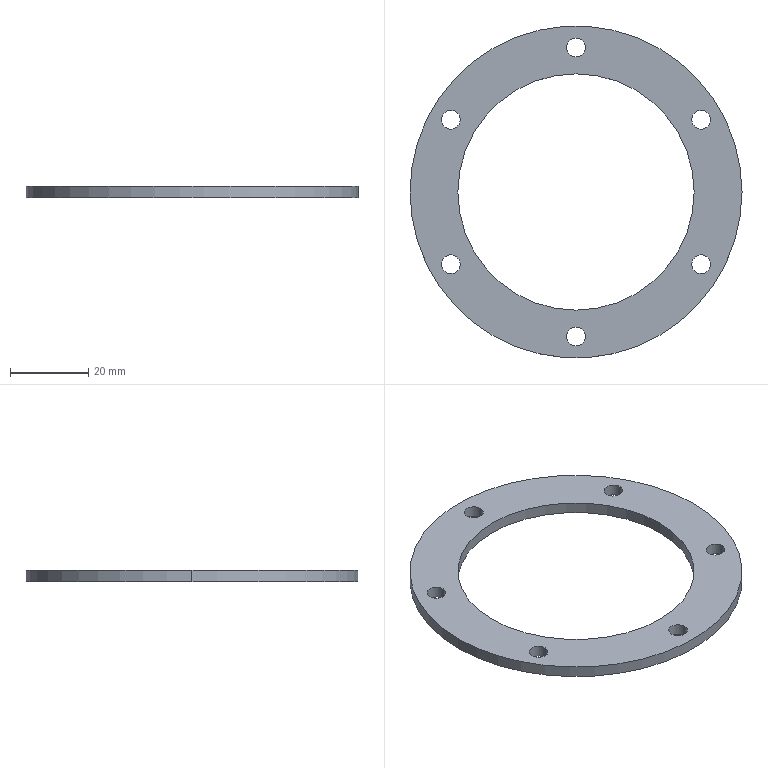Part | SolidWorks | features Extrusion 1, ICE 1 | 1 solid | 18 faces | box 85 x 85 x 3 mm | volume 8074 mm3 | cylinder 16 | plane 2 | commonest cylinder face diameters 4.8 x12 60.5 x2 85 x2
STEP:
#1=CARTESIAN_POINT('',(-34.443,18.5,0.));
#2=VERTEX_POINT('',#1);
#3=CARTESIAN_POINT('',(-29.643,18.5,0.));
#4=VERTEX_POINT('',#3);
#5=CARTESIAN_POINT('',(-32.043,18.5,0.));
#6=DIRECTION('',(0.,0.,1.));
#7=DIRECTION('',(1.,0.,0.));
#8=AXIS2_PLACEMENT_3D('',#5,#6,#7);
#9=CIRCLE('',#8,2.4);
#10=EDGE_CURVE('',#2,#4,#9,.T.);
#11=ORIENTED_EDGE('',*,*,#10,.F.);
#12=CARTESIAN_POINT('',(-34.443,18.5,3.));
#13=VERTEX_POINT('',#12);
#14=CARTESIAN_POINT('',(-34.443,18.5,0.));
#15=DIRECTION('',(0.,0.,1.));
#16=VECTOR('',#15,1000.);
#17=LINE('',#14,#16);
#18=EDGE_CURVE('',#2,#13,#17,.T.);
#19=ORIENTED_EDGE('',*,*,#18,.T.);
#20=CARTESIAN_POINT('',(-29.643,18.5,3.));
#21=VERTEX_POINT('',#20);
#22=CARTESIAN_POINT('',(-32.043,18.5,3.));
#23=DIRECTION('',(0.,0.,1.));
#24=DIRECTION('',(1.,0.,0.));
#25=AXIS2_PLACEMENT_3D('',#22,#23,#24);
#26=CIRCLE('',#25,2.4);
#27=EDGE_CURVE('',#13,#21,#26,.T.);
#28=ORIENTED_EDGE('',*,*,#27,.T.);
#29=CARTESIAN_POINT('',(-29.643,18.5,0.));
#30=DIRECTION('',(0.,0.,1.));
#31=VECTOR('',#30,1000.);
#32=LINE('',#29,#31);
#33=EDGE_CURVE('',#4,#21,#32,.T.);
#34=ORIENTED_EDGE('',*,*,#33,.F.);
#35=EDGE_LOOP('',(#11,#19,#28,#34));
#36=FACE_OUTER_BOUND('',#35,.T.);
#37=CARTESIAN_POINT('',(-32.043,18.5,0.));
#38=DIRECTION('',(0.,0.,1.));
#39=DIRECTION('',(1.,0.,0.));
#40=AXIS2_PLACEMENT_3D('',#37,#38,#39);
#41=CYLINDRICAL_SURFACE('',#40,2.4);
#42=ADVANCED_FACE('',(#36),#41,.F.);
#43=CARTESIAN_POINT('',(-34.443,-18.5,0.));
#44=VERTEX_POINT('',#43);
#45=CARTESIAN_POINT('',(-29.643,-18.5,0.));
#46=VERTEX_POINT('',#45);
#47=CARTESIAN_POINT('',(-32.043,-18.5,0.));
#48=DIRECTION('',(0.,0.,1.));
#49=DIRECTION('',(1.,0.,0.));
#50=AXIS2_PLACEMENT_3D('',#47,#48,#49);
#51=CIRCLE('',#50,2.4);
#52=EDGE_CURVE('',#44,#46,#51,.T.);
#53=ORIENTED_EDGE('',*,*,#52,.F.);
#54=CARTESIAN_POINT('',(-34.443,-18.5,3.));
#55=VERTEX_POINT('',#54);
#56=CARTESIAN_POINT('',(-34.443,-18.5,0.));
#57=DIRECTION('',(0.,0.,1.));
#58=VECTOR('',#57,1000.);
#59=LINE('',#56,#58);
#60=EDGE_CURVE('',#44,#55,#59,.T.);
#61=ORIENTED_EDGE('',*,*,#60,.T.);
#62=CARTESIAN_POINT('',(-29.643,-18.5,3.));
#63=VERTEX_POINT('',#62);
#64=CARTESIAN_POINT('',(-32.043,-18.5,3.));
#65=DIRECTION('',(0.,0.,1.));
#66=DIRECTION('',(1.,0.,0.));
#67=AXIS2_PLACEMENT_3D('',#64,#65,#66);
#68=CIRCLE('',#67,2.4);
#69=EDGE_CURVE('',#55,#63,#68,.T.);
#70=ORIENTED_EDGE('',*,*,#69,.T.);
#71=CARTESIAN_POINT('',(-29.643,-18.5,0.));
#72=DIRECTION('',(0.,0.,1.));
#73=VECTOR('',#72,1000.);
#74=LINE('',#71,#73);
#75=EDGE_CURVE('',#46,#63,#74,.T.);
#76=ORIENTED_EDGE('',*,*,#75,.F.);
#77=EDGE_LOOP('',(#53,#61,#70,#76));
#78=FACE_OUTER_BOUND('',#77,.T.);
#79=CARTESIAN_POINT('',(-32.043,-18.5,0.));
#80=DIRECTION('',(0.,0.,1.));
#81=DIRECTION('',(1.,0.,0.));
#82=AXIS2_PLACEMENT_3D('',#79,#80,#81);
#83=CYLINDRICAL_SURFACE('',#82,2.4);
#84=ADVANCED_FACE('',(#78),#83,.F.);
#85=CARTESIAN_POINT('',(-2.4,-37.,0.));
#86=VERTEX_POINT('',#85);
#87=CARTESIAN_POINT('',(2.4,-37.,0.));
#88=VERTEX_POINT('',#87);
#89=CARTESIAN_POINT('',(0.,-37.,0.));
#90=DIRECTION('',(0.,0.,1.));
#91=DIRECTION('',(1.,0.,0.));
#92=AXIS2_PLACEMENT_3D('',#89,#90,#91);
#93=CIRCLE('',#92,2.4);
#94=EDGE_CURVE('',#86,#88,#93,.T.);
#95=ORIENTED_EDGE('',*,*,#94,.F.);
#96=CARTESIAN_POINT('',(-2.4,-37.,3.));
#97=VERTEX_POINT('',#96);
#98=CARTESIAN_POINT('',(-2.4,-37.,0.));
#99=DIRECTION('',(0.,0.,1.));
#100=VECTOR('',#99,1000.);
#101=LINE('',#98,#100);
#102=EDGE_CURVE('',#86,#97,#101,.T.);
#103=ORIENTED_EDGE('',*,*,#102,.T.);
#104=CARTESIAN_POINT('',(2.4,-37.,3.));
#105=VERTEX_POINT('',#104);
#106=CARTESIAN_POINT('',(0.,-37.,3.));
#107=DIRECTION('',(0.,0.,1.));
#108=DIRECTION('',(1.,0.,0.));
#109=AXIS2_PLACEMENT_3D('',#106,#107,#108);
#110=CIRCLE('',#109,2.4);
#111=EDGE_CURVE('',#97,#105,#110,.T.);
#112=ORIENTED_EDGE('',*,*,#111,.T.);
#113=CARTESIAN_POINT('',(2.4,-37.,0.));
#114=DIRECTION('',(0.,0.,1.));
#115=VECTOR('',#114,1000.);
#116=LINE('',#113,#115);
#117=EDGE_CURVE('',#88,#105,#116,.T.);
#118=ORIENTED_EDGE('',*,*,#117,.F.);
#119=EDGE_LOOP('',(#95,#103,#112,#118));
#120=FACE_OUTER_BOUND('',#119,.T.);
#121=CARTESIAN_POINT('',(0.,-37.,0.));
#122=DIRECTION('',(0.,0.,1.));
#123=DIRECTION('',(1.,0.,0.));
#124=AXIS2_PLACEMENT_3D('',#121,#122,#123);
#125=CYLINDRICAL_SURFACE('',#124,2.4);
#126=ADVANCED_FACE('',(#120),#125,.F.);
#127=CARTESIAN_POINT('',(29.643,-18.5,0.));
#128=VERTEX_POINT('',#127);
#129=CARTESIAN_POINT('',(34.443,-18.5,0.));
#130=VERTEX_POINT('',#129);
#131=CARTESIAN_POINT('',(32.043,-18.5,0.));
#132=DIRECTION('',(0.,0.,1.));
#133=DIRECTION('',(1.,0.,0.));
#134=AXIS2_PLACEMENT_3D('',#131,#132,#133);
#135=CIRCLE('',#134,2.4);
#136=EDGE_CURVE('',#128,#130,#135,.T.);
#137=ORIENTED_EDGE('',*,*,#136,.F.);
#138=CARTESIAN_POINT('',(29.643,-18.5,3.));
#139=VERTEX_POINT('',#138);
#140=CARTESIAN_POINT('',(29.643,-18.5,0.));
#141=DIRECTION('',(0.,0.,1.));
#142=VECTOR('',#141,1000.);
#143=LINE('',#140,#142);
#144=EDGE_CURVE('',#128,#139,#143,.T.);
#145=ORIENTED_EDGE('',*,*,#144,.T.);
#146=CARTESIAN_POINT('',(34.443,-18.5,3.));
#147=VERTEX_POINT('',#146);
#148=CARTESIAN_POINT('',(32.043,-18.5,3.));
#149=DIRECTION('',(0.,0.,1.));
#150=DIRECTION('',(1.,0.,0.));
#151=AXIS2_PLACEMENT_3D('',#148,#149,#150);
#152=CIRCLE('',#151,2.4);
#153=EDGE_CURVE('',#139,#147,#152,.T.);
#154=ORIENTED_EDGE('',*,*,#153,.T.);
#155=CARTESIAN_POINT('',(34.443,-18.5,0.));
#156=DIRECTION('',(0.,0.,1.));
#157=VECTOR('',#156,1000.);
#158=LINE('',#155,#157);
#159=EDGE_CURVE('',#130,#147,#158,.T.);
#160=ORIENTED_EDGE('',*,*,#159,.F.);
#161=EDGE_LOOP('',(#137,#145,#154,#160));
#162=FACE_OUTER_BOUND('',#161,.T.);
#163=CARTESIAN_POINT('',(32.043,-18.5,0.));
#164=DIRECTION('',(0.,0.,1.));
#165=DIRECTION('',(1.,0.,0.));
#166=AXIS2_PLACEMENT_3D('',#163,#164,#165);
#167=CYLINDRICAL_SURFACE('',#166,2.4);
#168=ADVANCED_FACE('',(#162),#167,.F.);
#169=CARTESIAN_POINT('',(29.643,18.5,0.));
#170=VERTEX_POINT('',#169);
#171=CARTESIAN_POINT('',(34.443,18.5,0.));
#172=VERTEX_POINT('',#171);
#173=CARTESIAN_POINT('',(32.043,18.5,0.));
#174=DIRECTION('',(0.,0.,1.));
#175=DIRECTION('',(1.,0.,0.));
#176=AXIS2_PLACEMENT_3D('',#173,#174,#175);
#177=CIRCLE('',#176,2.4);
#178=EDGE_CURVE('',#170,#172,#177,.T.);
#179=ORIENTED_EDGE('',*,*,#178,.F.);
#180=CARTESIAN_POINT('',(29.643,18.5,3.));
#181=VERTEX_POINT('',#180);
#182=CARTESIAN_POINT('',(29.643,18.5,0.));
#183=DIRECTION('',(0.,0.,1.));
#184=VECTOR('',#183,1000.);
#185=LINE('',#182,#184);
#186=EDGE_CURVE('',#170,#181,#185,.T.);
#187=ORIENTED_EDGE('',*,*,#186,.T.);
#188=CARTESIAN_POINT('',(34.443,18.5,3.));
#189=VERTEX_POINT('',#188);
#190=CARTESIAN_POINT('',(32.043,18.5,3.));
#191=DIRECTION('',(0.,0.,1.));
#192=DIRECTION('',(1.,0.,0.));
#193=AXIS2_PLACEMENT_3D('',#190,#191,#192);
#194=CIRCLE('',#193,2.4);
#195=EDGE_CURVE('',#181,#189,#194,.T.);
#196=ORIENTED_EDGE('',*,*,#195,.T.);
#197=CARTESIAN_POINT('',(34.443,18.5,0.));
#198=DIRECTION('',(0.,0.,1.));
#199=VECTOR('',#198,1000.);
#200=LINE('',#197,#199);
#201=EDGE_CURVE('',#172,#189,#200,.T.);
#202=ORIENTED_EDGE('',*,*,#201,.F.);
#203=EDGE_LOOP('',(#179,#187,#196,#202));
#204=FACE_OUTER_BOUND('',#203,.T.);
#205=CARTESIAN_POINT('',(32.043,18.5,0.));
#206=DIRECTION('',(0.,0.,1.));
#207=DIRECTION('',(1.,0.,0.));
#208=AXIS2_PLACEMENT_3D('',#205,#206,#207);
#209=CYLINDRICAL_SURFACE('',#208,2.4);
#210=ADVANCED_FACE('',(#204),#209,.F.);
#211=CARTESIAN_POINT('',(-2.4,37.,0.));
#212=VERTEX_POINT('',#211);
#213=CARTESIAN_POINT('',(2.4,37.,0.));
#214=VERTEX_POINT('',#213);
#215=CARTESIAN_POINT('',(0.,37.,0.));
#216=DIRECTION('',(0.,0.,1.));
#217=DIRECTION('',(1.,0.,0.));
#218=AXIS2_PLACEMENT_3D('',#215,#216,#217);
#219=CIRCLE('',#218,2.4);
#220=EDGE_CURVE('',#212,#214,#219,.T.);
#221=ORIENTED_EDGE('',*,*,#220,.F.);
#222=CARTESIAN_POINT('',(-2.4,37.,3.));
#223=VERTEX_POINT('',#222);
#224=CARTESIAN_POINT('',(-2.4,37.,0.));
#225=DIRECTION('',(0.,0.,1.));
#226=VECTOR('',#225,1000.);
#227=LINE('',#224,#226);
#228=EDGE_CURVE('',#212,#223,#227,.T.);
#229=ORIENTED_EDGE('',*,*,#228,.T.);
#230=CARTESIAN_POINT('',(2.4,37.,3.));
#231=VERTEX_POINT('',#230);
#232=CARTESIAN_POINT('',(0.,37.,3.));
#233=DIRECTION('',(0.,0.,1.));
#234=DIRECTION('',(1.,0.,0.));
#235=AXIS2_PLACEMENT_3D('',#232,#233,#234);
#236=CIRCLE('',#235,2.4);
#237=EDGE_CURVE('',#223,#231,#236,.T.);
#238=ORIENTED_EDGE('',*,*,#237,.T.);
#239=CARTESIAN_POINT('',(2.4,37.,0.));
#240=DIRECTION('',(0.,0.,1.));
#241=VECTOR('',#240,1000.);
#242=LINE('',#239,#241);
#243=EDGE_CURVE('',#214,#231,#242,.T.);
#244=ORIENTED_EDGE('',*,*,#243,.F.);
#245=EDGE_LOOP('',(#221,#229,#238,#244));
#246=FACE_OUTER_BOUND('',#245,.T.);
#247=CARTESIAN_POINT('',(0.,37.,0.));
#248=DIRECTION('',(0.,0.,1.));
#249=DIRECTION('',(1.,0.,0.));
#250=AXIS2_PLACEMENT_3D('',#247,#248,#249);
#251=CYLINDRICAL_SURFACE('',#250,2.4);
#252=ADVANCED_FACE('',(#246),#251,.F.);
#253=CARTESIAN_POINT('',(-30.25,0.,3.));
#254=VERTEX_POINT('',#253);
#255=CARTESIAN_POINT('',(30.25,0.,3.));
#256=VERTEX_POINT('',#255);
#257=CARTESIAN_POINT('',(0.,0.,3.));
#258=DIRECTION('',(0.,0.,1.));
#259=DIRECTION('',(1.,0.,0.));
#260=AXIS2_PLACEMENT_3D('',#257,#258,#259);
#261=CIRCLE('',#260,30.25);
#262=EDGE_CURVE('',#254,#256,#261,.T.);
#263=ORIENTED_EDGE('',*,*,#262,.T.);
#264=CARTESIAN_POINT('',(30.25,0.,0.));
#265=VERTEX_POINT('',#264);
#266=CARTESIAN_POINT('',(30.25,0.,3.));
#267=DIRECTION('',(0.,0.,-1.));
#268=VECTOR('',#267,1000.);
#269=LINE('',#266,#268);
#270=EDGE_CURVE('',#256,#265,#269,.T.);
#271=ORIENTED_EDGE('',*,*,#270,.T.);
#272=CARTESIAN_POINT('',(-30.25,0.,0.));
#273=VERTEX_POINT('',#272);
#274=CARTESIAN_POINT('',(0.,0.,0.));
#275=DIRECTION('',(0.,0.,1.));
#276=DIRECTION('',(1.,0.,0.));
#277=AXIS2_PLACEMENT_3D('',#274,#275,#276);
#278=CIRCLE('',#277,30.25);
#279=EDGE_CURVE('',#273,#265,#278,.T.);
#280=ORIENTED_EDGE('',*,*,#279,.F.);
#281=CARTESIAN_POINT('',(-30.25,0.,3.));
#282=DIRECTION('',(0.,0.,-1.));
#283=VECTOR('',#282,1000.);
#284=LINE('',#281,#283);
#285=EDGE_CURVE('',#254,#273,#284,.T.);
#286=ORIENTED_EDGE('',*,*,#285,.F.);
#287=EDGE_LOOP('',(#263,#271,#280,#286));
#288=FACE_OUTER_BOUND('',#287,.T.);
#289=CARTESIAN_POINT('',(0.,0.,3.));
#290=DIRECTION('',(0.,0.,-1.));
#291=DIRECTION('',(-1.,0.,0.));
#292=AXIS2_PLACEMENT_3D('',#289,#290,#291);
#293=CYLINDRICAL_SURFACE('',#292,30.25);
#294=ADVANCED_FACE('',(#288),#293,.F.);
#295=CARTESIAN_POINT('',(42.5,0.,3.));
#296=VERTEX_POINT('',#295);
#297=CARTESIAN_POINT('',(-42.5,0.,3.));
#298=VERTEX_POINT('',#297);
#299=CARTESIAN_POINT('',(0.,0.,3.));
#300=DIRECTION('',(0.,0.,1.));
#301=DIRECTION('',(1.,0.,0.));
#302=AXIS2_PLACEMENT_3D('',#299,#300,#301);
#303=CIRCLE('',#302,42.5);
#304=EDGE_CURVE('',#296,#298,#303,.T.);
#305=ORIENTED_EDGE('',*,*,#304,.F.);
#306=CARTESIAN_POINT('',(42.5,0.,0.));
#307=VERTEX_POINT('',#306);
#308=CARTESIAN_POINT('',(42.5,0.,3.));
#309=DIRECTION('',(0.,0.,-1.));
#310=VECTOR('',#309,1000.);
#311=LINE('',#308,#310);
#312=EDGE_CURVE('',#296,#307,#311,.T.);
#313=ORIENTED_EDGE('',*,*,#312,.T.);
#314=CARTESIAN_POINT('',(-42.5,0.,0.));
#315=VERTEX_POINT('',#314);
#316=CARTESIAN_POINT('',(0.,0.,0.));
#317=DIRECTION('',(0.,0.,1.));
#318=DIRECTION('',(1.,0.,0.));
#319=AXIS2_PLACEMENT_3D('',#316,#317,#318);
#320=CIRCLE('',#319,42.5);
#321=EDGE_CURVE('',#307,#315,#320,.T.);
#322=ORIENTED_EDGE('',*,*,#321,.T.);
#323=CARTESIAN_POINT('',(-42.5,0.,3.));
#324=DIRECTION('',(0.,0.,-1.));
#325=VECTOR('',#324,1000.);
#326=LINE('',#323,#325);
#327=EDGE_CURVE('',#298,#315,#326,.T.);
#328=ORIENTED_EDGE('',*,*,#327,.F.);
#329=EDGE_LOOP('',(#305,#313,#322,#328));
#330=FACE_OUTER_BOUND('',#329,.T.);
#331=CARTESIAN_POINT('',(0.,0.,3.));
#332=DIRECTION('',(0.,0.,-1.));
#333=DIRECTION('',(-1.,0.,0.));
#334=AXIS2_PLACEMENT_3D('',#331,#332,#333);
#335=CYLINDRICAL_SURFACE('',#334,42.5);
#336=ADVANCED_FACE('',(#330),#335,.T.);
#337=CARTESIAN_POINT('',(-32.043,18.5,3.));
#338=DIRECTION('',(0.,0.,1.));
#339=DIRECTION('',(1.,0.,0.));
#340=AXIS2_PLACEMENT_3D('',#337,#338,#339);
#341=CIRCLE('',#340,2.4);
#342=EDGE_CURVE('',#21,#13,#341,.T.);
#343=ORIENTED_EDGE('',*,*,#342,.F.);
#344=ORIENTED_EDGE('',*,*,#27,.F.);
#345=EDGE_LOOP('',(#343,#344));
#346=FACE_BOUND('',#345,.T.);
#347=CARTESIAN_POINT('',(-32.043,-18.5,3.));
#348=DIRECTION('',(0.,0.,1.));
#349=DIRECTION('',(1.,0.,0.));
#350=AXIS2_PLACEMENT_3D('',#347,#348,#349);
#351=CIRCLE('',#350,2.4);
#352=EDGE_CURVE('',#63,#55,#351,.T.);
#353=ORIENTED_EDGE('',*,*,#352,.F.);
#354=ORIENTED_EDGE('',*,*,#69,.F.);
#355=EDGE_LOOP('',(#353,#354));
#356=FACE_BOUND('',#355,.T.);
#357=CARTESIAN_POINT('',(0.,-37.,3.));
#358=DIRECTION('',(0.,0.,1.));
#359=DIRECTION('',(1.,0.,0.));
#360=AXIS2_PLACEMENT_3D('',#357,#358,#359);
#361=CIRCLE('',#360,2.4);
#362=EDGE_CURVE('',#105,#97,#361,.T.);
#363=ORIENTED_EDGE('',*,*,#362,.F.);
#364=ORIENTED_EDGE('',*,*,#111,.F.);
#365=EDGE_LOOP('',(#363,#364));
#366=FACE_BOUND('',#365,.T.);
#367=CARTESIAN_POINT('',(32.043,-18.5,3.));
#368=DIRECTION('',(0.,0.,1.));
#369=DIRECTION('',(1.,0.,0.));
#370=AXIS2_PLACEMENT_3D('',#367,#368,#369);
#371=CIRCLE('',#370,2.4);
#372=EDGE_CURVE('',#147,#139,#371,.T.);
#373=ORIENTED_EDGE('',*,*,#372,.F.);
#374=ORIENTED_EDGE('',*,*,#153,.F.);
#375=EDGE_LOOP('',(#373,#374));
#376=FACE_BOUND('',#375,.T.);
#377=CARTESIAN_POINT('',(32.043,18.5,3.));
#378=DIRECTION('',(0.,0.,1.));
#379=DIRECTION('',(1.,0.,0.));
#380=AXIS2_PLACEMENT_3D('',#377,#378,#379);
#381=CIRCLE('',#380,2.4);
#382=EDGE_CURVE('',#189,#181,#381,.T.);
#383=ORIENTED_EDGE('',*,*,#382,.F.);
#384=ORIENTED_EDGE('',*,*,#195,.F.);
#385=EDGE_LOOP('',(#383,#384));
#386=FACE_BOUND('',#385,.T.);
#387=CARTESIAN_POINT('',(0.,37.,3.));
#388=DIRECTION('',(0.,0.,1.));
#389=DIRECTION('',(1.,0.,0.));
#390=AXIS2_PLACEMENT_3D('',#387,#388,#389);
#391=CIRCLE('',#390,2.4);
#392=EDGE_CURVE('',#231,#223,#391,.T.);
#393=ORIENTED_EDGE('',*,*,#392,.F.);
#394=ORIENTED_EDGE('',*,*,#237,.F.);
#395=EDGE_LOOP('',(#393,#394));
#396=FACE_BOUND('',#395,.T.);
#397=CARTESIAN_POINT('',(0.,0.,3.));
#398=DIRECTION('',(0.,0.,1.));
#399=DIRECTION('',(1.,0.,0.));
#400=AXIS2_PLACEMENT_3D('',#397,#398,#399);
#401=CIRCLE('',#400,42.5);
#402=EDGE_CURVE('',#298,#296,#401,.T.);
#403=ORIENTED_EDGE('',*,*,#402,.T.);
#404=ORIENTED_EDGE('',*,*,#304,.T.);
#405=EDGE_LOOP('',(#403,#404));
#406=FACE_OUTER_BOUND('',#405,.T.);
#407=ORIENTED_EDGE('',*,*,#262,.F.);
#408=CARTESIAN_POINT('',(0.,0.,3.));
#409=DIRECTION('',(0.,0.,1.));
#410=DIRECTION('',(1.,0.,0.));
#411=AXIS2_PLACEMENT_3D('',#408,#409,#410);
#412=CIRCLE('',#411,30.25);
#413=EDGE_CURVE('',#256,#254,#412,.T.);
#414=ORIENTED_EDGE('',*,*,#413,.F.);
#415=EDGE_LOOP('',(#407,#414));
#416=FACE_BOUND('',#415,.T.);
#417=CARTESIAN_POINT('',(0.,0.,3.));
#418=DIRECTION('',(0.,0.,1.));
#419=DIRECTION('',(1.,0.,0.));
#420=AXIS2_PLACEMENT_3D('',#417,#418,#419);
#421=PLANE('',#420);
#422=ADVANCED_FACE('',(#346,#356,#366,#376,#386,#396,#406,#416),#421,.T.);
#423=CARTESIAN_POINT('',(-32.043,18.5,0.));
#424=DIRECTION('',(0.,0.,1.));
#425=DIRECTION('',(1.,0.,0.));
#426=AXIS2_PLACEMENT_3D('',#423,#424,#425);
#427=CIRCLE('',#426,2.4);
#428=EDGE_CURVE('',#4,#2,#427,.T.);
#429=ORIENTED_EDGE('',*,*,#428,.T.);
#430=ORIENTED_EDGE('',*,*,#10,.T.);
#431=EDGE_LOOP('',(#429,#430));
#432=FACE_BOUND('',#431,.T.);
#433=CARTESIAN_POINT('',(-32.043,-18.5,0.));
#434=DIRECTION('',(0.,0.,1.));
#435=DIRECTION('',(1.,0.,0.));
#436=AXIS2_PLACEMENT_3D('',#433,#434,#435);
#437=CIRCLE('',#436,2.4);
#438=EDGE_CURVE('',#46,#44,#437,.T.);
#439=ORIENTED_EDGE('',*,*,#438,.T.);
#440=ORIENTED_EDGE('',*,*,#52,.T.);
#441=EDGE_LOOP('',(#439,#440));
#442=FACE_BOUND('',#441,.T.);
#443=CARTESIAN_POINT('',(0.,-37.,0.));
#444=DIRECTION('',(0.,0.,1.));
#445=DIRECTION('',(1.,0.,0.));
#446=AXIS2_PLACEMENT_3D('',#443,#444,#445);
#447=CIRCLE('',#446,2.4);
#448=EDGE_CURVE('',#88,#86,#447,.T.);
#449=ORIENTED_EDGE('',*,*,#448,.T.);
#450=ORIENTED_EDGE('',*,*,#94,.T.);
#451=EDGE_LOOP('',(#449,#450));
#452=FACE_BOUND('',#451,.T.);
#453=CARTESIAN_POINT('',(32.043,-18.5,0.));
#454=DIRECTION('',(0.,0.,1.));
#455=DIRECTION('',(1.,0.,0.));
#456=AXIS2_PLACEMENT_3D('',#453,#454,#455);
#457=CIRCLE('',#456,2.4);
#458=EDGE_CURVE('',#130,#128,#457,.T.);
#459=ORIENTED_EDGE('',*,*,#458,.T.);
#460=ORIENTED_EDGE('',*,*,#136,.T.);
#461=EDGE_LOOP('',(#459,#460));
#462=FACE_BOUND('',#461,.T.);
#463=CARTESIAN_POINT('',(32.043,18.5,0.));
#464=DIRECTION('',(0.,0.,1.));
#465=DIRECTION('',(1.,0.,0.));
#466=AXIS2_PLACEMENT_3D('',#463,#464,#465);
#467=CIRCLE('',#466,2.4);
#468=EDGE_CURVE('',#172,#170,#467,.T.);
#469=ORIENTED_EDGE('',*,*,#468,.T.);
#470=ORIENTED_EDGE('',*,*,#178,.T.);
#471=EDGE_LOOP('',(#469,#470));
#472=FACE_BOUND('',#471,.T.);
#473=CARTESIAN_POINT('',(0.,37.,0.));
#474=DIRECTION('',(0.,0.,1.));
#475=DIRECTION('',(1.,0.,0.));
#476=AXIS2_PLACEMENT_3D('',#473,#474,#475);
#477=CIRCLE('',#476,2.4);
#478=EDGE_CURVE('',#214,#212,#477,.T.);
#479=ORIENTED_EDGE('',*,*,#478,.T.);
#480=ORIENTED_EDGE('',*,*,#220,.T.);
#481=EDGE_LOOP('',(#479,#480));
#482=FACE_BOUND('',#481,.T.);
#483=CARTESIAN_POINT('',(0.,0.,0.));
#484=DIRECTION('',(0.,0.,1.));
#485=DIRECTION('',(1.,0.,0.));
#486=AXIS2_PLACEMENT_3D('',#483,#484,#485);
#487=CIRCLE('',#486,42.5);
#488=EDGE_CURVE('',#315,#307,#487,.T.);
#489=ORIENTED_EDGE('',*,*,#488,.F.);
#490=ORIENTED_EDGE('',*,*,#321,.F.);
#491=EDGE_LOOP('',(#489,#490));
#492=FACE_OUTER_BOUND('',#491,.T.);
#493=ORIENTED_EDGE('',*,*,#279,.T.);
#494=CARTESIAN_POINT('',(0.,0.,0.));
#495=DIRECTION('',(0.,0.,1.));
#496=DIRECTION('',(1.,0.,0.));
#497=AXIS2_PLACEMENT_3D('',#494,#495,#496);
#498=CIRCLE('',#497,30.25);
#499=EDGE_CURVE('',#265,#273,#498,.T.);
#500=ORIENTED_EDGE('',*,*,#499,.T.);
#501=EDGE_LOOP('',(#493,#500));
#502=FACE_BOUND('',#501,.T.);
#503=CARTESIAN_POINT('',(0.,0.,0.));
#504=DIRECTION('',(0.,0.,1.));
#505=DIRECTION('',(1.,0.,0.));
#506=AXIS2_PLACEMENT_3D('',#503,#504,#505);
#507=PLANE('',#506);
#508=ADVANCED_FACE('',(#432,#442,#452,#462,#472,#482,#492,#502),#507,.F.);
#509=ORIENTED_EDGE('',*,*,#312,.F.);
#510=ORIENTED_EDGE('',*,*,#402,.F.);
#511=ORIENTED_EDGE('',*,*,#327,.T.);
#512=ORIENTED_EDGE('',*,*,#488,.T.);
#513=EDGE_LOOP('',(#509,#510,#511,#512));
#514=FACE_OUTER_BOUND('',#513,.T.);
#515=CARTESIAN_POINT('',(0.,0.,3.));
#516=DIRECTION('',(0.,0.,-1.));
#517=DIRECTION('',(-1.,0.,0.));
#518=AXIS2_PLACEMENT_3D('',#515,#516,#517);
#519=CYLINDRICAL_SURFACE('',#518,42.5);
#520=ADVANCED_FACE('',(#514),#519,.T.);
#521=ORIENTED_EDGE('',*,*,#270,.F.);
#522=ORIENTED_EDGE('',*,*,#413,.T.);
#523=ORIENTED_EDGE('',*,*,#285,.T.);
#524=ORIENTED_EDGE('',*,*,#499,.F.);
#525=EDGE_LOOP('',(#521,#522,#523,#524));
#526=FACE_OUTER_BOUND('',#525,.T.);
#527=CARTESIAN_POINT('',(0.,0.,3.));
#528=DIRECTION('',(0.,0.,-1.));
#529=DIRECTION('',(-1.,0.,0.));
#530=AXIS2_PLACEMENT_3D('',#527,#528,#529);
#531=CYLINDRICAL_SURFACE('',#530,30.25);
#532=ADVANCED_FACE('',(#526),#531,.F.);
#533=ORIENTED_EDGE('',*,*,#228,.F.);
#534=ORIENTED_EDGE('',*,*,#478,.F.);
#535=ORIENTED_EDGE('',*,*,#243,.T.);
#536=ORIENTED_EDGE('',*,*,#392,.T.);
#537=EDGE_LOOP('',(#533,#534,#535,#536));
#538=FACE_OUTER_BOUND('',#537,.T.);
#539=CARTESIAN_POINT('',(0.,37.,0.));
#540=DIRECTION('',(0.,0.,1.));
#541=DIRECTION('',(1.,0.,0.));
#542=AXIS2_PLACEMENT_3D('',#539,#540,#541);
#543=CYLINDRICAL_SURFACE('',#542,2.4);
#544=ADVANCED_FACE('',(#538),#543,.F.);
#545=ORIENTED_EDGE('',*,*,#186,.F.);
#546=ORIENTED_EDGE('',*,*,#468,.F.);
#547=ORIENTED_EDGE('',*,*,#201,.T.);
#548=ORIENTED_EDGE('',*,*,#382,.T.);
#549=EDGE_LOOP('',(#545,#546,#547,#548));
#550=FACE_OUTER_BOUND('',#549,.T.);
#551=CARTESIAN_POINT('',(32.043,18.5,0.));
#552=DIRECTION('',(0.,0.,1.));
#553=DIRECTION('',(1.,0.,0.));
#554=AXIS2_PLACEMENT_3D('',#551,#552,#553);
#555=CYLINDRICAL_SURFACE('',#554,2.4);
#556=ADVANCED_FACE('',(#550),#555,.F.);
#557=ORIENTED_EDGE('',*,*,#144,.F.);
#558=ORIENTED_EDGE('',*,*,#458,.F.);
#559=ORIENTED_EDGE('',*,*,#159,.T.);
#560=ORIENTED_EDGE('',*,*,#372,.T.);
#561=EDGE_LOOP('',(#557,#558,#559,#560));
#562=FACE_OUTER_BOUND('',#561,.T.);
#563=CARTESIAN_POINT('',(32.043,-18.5,0.));
#564=DIRECTION('',(0.,0.,1.));
#565=DIRECTION('',(1.,0.,0.));
#566=AXIS2_PLACEMENT_3D('',#563,#564,#565);
#567=CYLINDRICAL_SURFACE('',#566,2.4);
#568=ADVANCED_FACE('',(#562),#567,.F.);
#569=ORIENTED_EDGE('',*,*,#102,.F.);
#570=ORIENTED_EDGE('',*,*,#448,.F.);
#571=ORIENTED_EDGE('',*,*,#117,.T.);
#572=ORIENTED_EDGE('',*,*,#362,.T.);
#573=EDGE_LOOP('',(#569,#570,#571,#572));
#574=FACE_OUTER_BOUND('',#573,.T.);
#575=CARTESIAN_POINT('',(0.,-37.,0.));
#576=DIRECTION('',(0.,0.,1.));
#577=DIRECTION('',(1.,0.,0.));
#578=AXIS2_PLACEMENT_3D('',#575,#576,#577);
#579=CYLINDRICAL_SURFACE('',#578,2.4);
#580=ADVANCED_FACE('',(#574),#579,.F.);
#581=ORIENTED_EDGE('',*,*,#60,.F.);
#582=ORIENTED_EDGE('',*,*,#438,.F.);
#583=ORIENTED_EDGE('',*,*,#75,.T.);
#584=ORIENTED_EDGE('',*,*,#352,.T.);
#585=EDGE_LOOP('',(#581,#582,#583,#584));
#586=FACE_OUTER_BOUND('',#585,.T.);
#587=CARTESIAN_POINT('',(-32.043,-18.5,0.));
#588=DIRECTION('',(0.,0.,1.));
#589=DIRECTION('',(1.,0.,0.));
#590=AXIS2_PLACEMENT_3D('',#587,#588,#589);
#591=CYLINDRICAL_SURFACE('',#590,2.4);
#592=ADVANCED_FACE('',(#586),#591,.F.);
#593=ORIENTED_EDGE('',*,*,#18,.F.);
#594=ORIENTED_EDGE('',*,*,#428,.F.);
#595=ORIENTED_EDGE('',*,*,#33,.T.);
#596=ORIENTED_EDGE('',*,*,#342,.T.);
#597=EDGE_LOOP('',(#593,#594,#595,#596));
#598=FACE_OUTER_BOUND('',#597,.T.);
#599=CARTESIAN_POINT('',(-32.043,18.5,0.));
#600=DIRECTION('',(0.,0.,1.));
#601=DIRECTION('',(1.,0.,0.));
#602=AXIS2_PLACEMENT_3D('',#599,#600,#601);
#603=CYLINDRICAL_SURFACE('',#602,2.4);
#604=ADVANCED_FACE('',(#598),#603,.F.);
#605=CLOSED_SHELL('',(#42,#84,#126,#168,#210,#252,#294,#336,#422,#508,#520,#532,#544,#556,#568,#580,#592,#604));
#606=MANIFOLD_SOLID_BREP('',#605);
#607=CARTESIAN_POINT('',(0.,0.,0.));
#608=DIRECTION('',(0.,0.,1.));
#609=DIRECTION('',(1.,0.,0.));
#610=AXIS2_PLACEMENT_3D('',#607,#608,#609);
#611=(LENGTH_UNIT()NAMED_UNIT(*)SI_UNIT(.MILLI.,.METRE.));
#612=UNCERTAINTY_MEASURE_WITH_UNIT(LENGTH_MEASURE(0.00001),#611,'','');
#613=(NAMED_UNIT(*)PLANE_ANGLE_UNIT()SI_UNIT($,.RADIAN.));
#614=(NAMED_UNIT(*)SI_UNIT($,.STERADIAN.)SOLID_ANGLE_UNIT());
#615=(GEOMETRIC_REPRESENTATION_CONTEXT(3)GLOBAL_UNCERTAINTY_ASSIGNED_CONTEXT((#612))GLOBAL_UNIT_ASSIGNED_CONTEXT((#611,#613,#614))REPRESENTATION_CONTEXT('',''));
#616=ADVANCED_BREP_SHAPE_REPRESENTATION('',(#606,#610),#615);